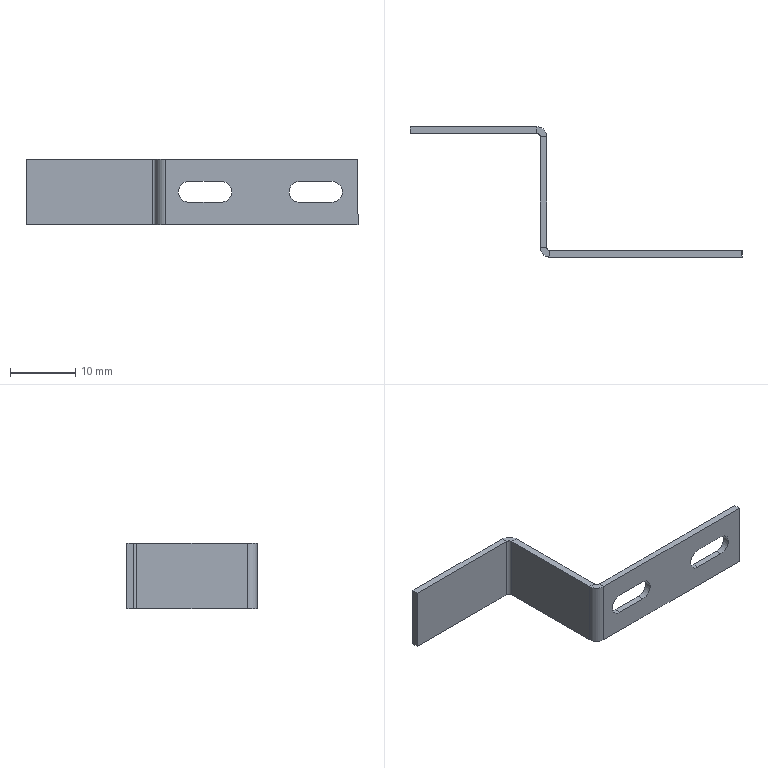Part | SolidWorks | features EdgeFlange 1, FlatPattern 1, ICE 1, SMBaseFlange 1, SheetMetal 1 | 1 solid | 30 faces | box 51 x 20 x 10 mm | volume 643.331 mm3 | plane 22 | cylinder 8 | commonest cylinder face diameters 3.2 x4 1 x2 3 x2
STEP:
#1=CARTESIAN_POINT('',(-1.,17.5,0.));
#2=VERTEX_POINT('',#1);
#3=CARTESIAN_POINT('',(-1.,0.5,0.));
#4=VERTEX_POINT('',#3);
#5=CARTESIAN_POINT('',(-1.,0.,0.));
#6=DIRECTION('',(0.,-1.,0.));
#7=VECTOR('',#6,1000.);
#8=LINE('',#5,#7);
#9=EDGE_CURVE('',#2,#4,#8,.T.);
#10=ORIENTED_EDGE('',*,*,#9,.F.);
#11=CARTESIAN_POINT('',(0.,17.5,0.));
#12=VERTEX_POINT('',#11);
#13=CARTESIAN_POINT('',(-1.,17.5,0.));
#14=DIRECTION('',(1.,0.,0.));
#15=VECTOR('',#14,1000.);
#16=LINE('',#13,#15);
#17=EDGE_CURVE('',#2,#12,#16,.T.);
#18=ORIENTED_EDGE('',*,*,#17,.T.);
#19=CARTESIAN_POINT('',(0.,0.5,0.));
#20=VERTEX_POINT('',#19);
#21=CARTESIAN_POINT('',(0.,0.,0.));
#22=DIRECTION('',(0.,-1.,0.));
#23=VECTOR('',#22,1000.);
#24=LINE('',#21,#23);
#25=EDGE_CURVE('',#12,#20,#24,.T.);
#26=ORIENTED_EDGE('',*,*,#25,.T.);
#27=CARTESIAN_POINT('',(0.,0.5,0.));
#28=DIRECTION('',(-1.,0.,0.));
#29=VECTOR('',#28,1000.);
#30=LINE('',#27,#29);
#31=EDGE_CURVE('',#20,#4,#30,.T.);
#32=ORIENTED_EDGE('',*,*,#31,.T.);
#33=EDGE_LOOP('',(#10,#18,#26,#32));
#34=FACE_OUTER_BOUND('',#33,.T.);
#35=CARTESIAN_POINT('',(0.5,-1.,0.));
#36=DIRECTION('',(0.,0.,-1.));
#37=DIRECTION('',(-1.,0.,0.));
#38=AXIS2_PLACEMENT_3D('',#35,#36,#37);
#39=PLANE('',#38);
#40=ADVANCED_FACE('',(#34),#39,.T.);
#41=ORIENTED_EDGE('',*,*,#25,.F.);
#42=CARTESIAN_POINT('',(0.,17.5,10.));
#43=VERTEX_POINT('',#42);
#44=CARTESIAN_POINT('',(0.,17.5,0.));
#45=DIRECTION('',(0.,0.,1.));
#46=VECTOR('',#45,1000.);
#47=LINE('',#44,#46);
#48=EDGE_CURVE('',#12,#43,#47,.T.);
#49=ORIENTED_EDGE('',*,*,#48,.T.);
#50=CARTESIAN_POINT('',(0.,0.5,10.));
#51=VERTEX_POINT('',#50);
#52=CARTESIAN_POINT('',(0.,0.,10.));
#53=DIRECTION('',(0.,-1.,0.));
#54=VECTOR('',#53,1000.);
#55=LINE('',#52,#54);
#56=EDGE_CURVE('',#43,#51,#55,.T.);
#57=ORIENTED_EDGE('',*,*,#56,.T.);
#58=CARTESIAN_POINT('',(0.,0.5,10.));
#59=DIRECTION('',(0.,0.,-1.));
#60=VECTOR('',#59,1000.);
#61=LINE('',#58,#60);
#62=EDGE_CURVE('',#51,#20,#61,.T.);
#63=ORIENTED_EDGE('',*,*,#62,.T.);
#64=EDGE_LOOP('',(#41,#49,#57,#63));
#65=FACE_OUTER_BOUND('',#64,.T.);
#66=CARTESIAN_POINT('',(0.,0.,10.));
#67=DIRECTION('',(1.,0.,0.));
#68=DIRECTION('',(0.,0.,-1.));
#69=AXIS2_PLACEMENT_3D('',#66,#67,#68);
#70=PLANE('',#69);
#71=ADVANCED_FACE('',(#65),#70,.T.);
#72=CARTESIAN_POINT('',(-1.,17.5,10.));
#73=VERTEX_POINT('',#72);
#74=CARTESIAN_POINT('',(-1.,17.5,0.));
#75=DIRECTION('',(0.,0.,1.));
#76=VECTOR('',#75,1000.);
#77=LINE('',#74,#76);
#78=EDGE_CURVE('',#2,#73,#77,.T.);
#79=ORIENTED_EDGE('',*,*,#78,.F.);
#80=ORIENTED_EDGE('',*,*,#9,.T.);
#81=CARTESIAN_POINT('',(-1.,0.5,10.));
#82=VERTEX_POINT('',#81);
#83=CARTESIAN_POINT('',(-1.,0.5,10.));
#84=DIRECTION('',(0.,0.,-1.));
#85=VECTOR('',#84,1000.);
#86=LINE('',#83,#85);
#87=EDGE_CURVE('',#82,#4,#86,.T.);
#88=ORIENTED_EDGE('',*,*,#87,.F.);
#89=CARTESIAN_POINT('',(-1.,0.,10.));
#90=DIRECTION('',(0.,-1.,0.));
#91=VECTOR('',#90,1000.);
#92=LINE('',#89,#91);
#93=EDGE_CURVE('',#73,#82,#92,.T.);
#94=ORIENTED_EDGE('',*,*,#93,.F.);
#95=EDGE_LOOP('',(#79,#80,#88,#94));
#96=FACE_OUTER_BOUND('',#95,.T.);
#97=CARTESIAN_POINT('',(-1.,0.,10.));
#98=DIRECTION('',(1.,0.,0.));
#99=DIRECTION('',(0.,0.,-1.));
#100=AXIS2_PLACEMENT_3D('',#97,#98,#99);
#101=PLANE('',#100);
#102=ADVANCED_FACE('',(#96),#101,.F.);
#103=CARTESIAN_POINT('',(-1.,17.5,10.));
#104=DIRECTION('',(1.,0.,0.));
#105=VECTOR('',#104,1000.);
#106=LINE('',#103,#105);
#107=EDGE_CURVE('',#73,#43,#106,.T.);
#108=ORIENTED_EDGE('',*,*,#107,.F.);
#109=ORIENTED_EDGE('',*,*,#93,.T.);
#110=CARTESIAN_POINT('',(-1.,0.5,10.));
#111=DIRECTION('',(1.,0.,0.));
#112=VECTOR('',#111,1000.);
#113=LINE('',#110,#112);
#114=EDGE_CURVE('',#82,#51,#113,.T.);
#115=ORIENTED_EDGE('',*,*,#114,.T.);
#116=ORIENTED_EDGE('',*,*,#56,.F.);
#117=EDGE_LOOP('',(#108,#109,#115,#116));
#118=FACE_OUTER_BOUND('',#117,.T.);
#119=CARTESIAN_POINT('',(0.5,0.5,10.));
#120=DIRECTION('',(0.,0.,-1.));
#121=DIRECTION('',(-1.,0.,0.));
#122=AXIS2_PLACEMENT_3D('',#119,#120,#121);
#123=PLANE('',#122);
#124=ADVANCED_FACE('',(#118),#123,.F.);
#125=CARTESIAN_POINT('',(0.5,0.,10.));
#126=VERTEX_POINT('',#125);
#127=CARTESIAN_POINT('',(0.5,-1.,10.));
#128=VERTEX_POINT('',#127);
#129=CARTESIAN_POINT('',(0.5,0.,10.));
#130=DIRECTION('',(0.,-1.,0.));
#131=VECTOR('',#130,1000.);
#132=LINE('',#129,#131);
#133=EDGE_CURVE('',#126,#128,#132,.T.);
#134=ORIENTED_EDGE('',*,*,#133,.F.);
#135=CARTESIAN_POINT('',(0.5,0.5,10.));
#136=DIRECTION('',(0.,0.,1.));
#137=DIRECTION('',(-1.,0.,0.));
#138=AXIS2_PLACEMENT_3D('',#135,#136,#137);
#139=CIRCLE('',#138,0.5);
#140=EDGE_CURVE('',#51,#126,#139,.T.);
#141=ORIENTED_EDGE('',*,*,#140,.F.);
#142=ORIENTED_EDGE('',*,*,#114,.F.);
#143=CARTESIAN_POINT('',(0.5,0.5,10.));
#144=DIRECTION('',(0.,0.,1.));
#145=DIRECTION('',(1.,0.,0.));
#146=AXIS2_PLACEMENT_3D('',#143,#144,#145);
#147=CIRCLE('',#146,1.5);
#148=EDGE_CURVE('',#82,#128,#147,.T.);
#149=ORIENTED_EDGE('',*,*,#148,.T.);
#150=EDGE_LOOP('',(#134,#141,#142,#149));
#151=FACE_OUTER_BOUND('',#150,.T.);
#152=CARTESIAN_POINT('',(0.5,0.,10.));
#153=DIRECTION('',(0.,0.,1.));
#154=DIRECTION('',(1.,0.,0.));
#155=AXIS2_PLACEMENT_3D('',#152,#153,#154);
#156=PLANE('',#155);
#157=ADVANCED_FACE('',(#151),#156,.T.);
#158=CARTESIAN_POINT('',(30.,0.,10.));
#159=VERTEX_POINT('',#158);
#160=CARTESIAN_POINT('',(0.,0.,10.));
#161=DIRECTION('',(1.,0.,0.));
#162=VECTOR('',#161,1000.);
#163=LINE('',#160,#162);
#164=EDGE_CURVE('',#126,#159,#163,.T.);
#165=ORIENTED_EDGE('',*,*,#164,.F.);
#166=ORIENTED_EDGE('',*,*,#133,.T.);
#167=CARTESIAN_POINT('',(30.,-1.,10.));
#168=VERTEX_POINT('',#167);
#169=CARTESIAN_POINT('',(0.,-1.,10.));
#170=DIRECTION('',(1.,0.,0.));
#171=VECTOR('',#170,1000.);
#172=LINE('',#169,#171);
#173=EDGE_CURVE('',#128,#168,#172,.T.);
#174=ORIENTED_EDGE('',*,*,#173,.T.);
#175=CARTESIAN_POINT('',(30.,0.,10.));
#176=DIRECTION('',(0.,-1.,0.));
#177=VECTOR('',#176,1000.);
#178=LINE('',#175,#177);
#179=EDGE_CURVE('',#159,#168,#178,.T.);
#180=ORIENTED_EDGE('',*,*,#179,.F.);
#181=EDGE_LOOP('',(#165,#166,#174,#180));
#182=FACE_OUTER_BOUND('',#181,.T.);
#183=CARTESIAN_POINT('',(-1.,0.5,10.));
#184=DIRECTION('',(0.,0.,1.));
#185=DIRECTION('',(1.,0.,0.));
#186=AXIS2_PLACEMENT_3D('',#183,#184,#185);
#187=PLANE('',#186);
#188=ADVANCED_FACE('',(#182),#187,.T.);
#189=ORIENTED_EDGE('',*,*,#31,.F.);
#190=CARTESIAN_POINT('',(0.5,0.,0.));
#191=VERTEX_POINT('',#190);
#192=CARTESIAN_POINT('',(0.5,0.5,0.));
#193=DIRECTION('',(0.,0.,1.));
#194=DIRECTION('',(-1.,0.,0.));
#195=AXIS2_PLACEMENT_3D('',#192,#193,#194);
#196=CIRCLE('',#195,0.5);
#197=EDGE_CURVE('',#20,#191,#196,.T.);
#198=ORIENTED_EDGE('',*,*,#197,.T.);
#199=CARTESIAN_POINT('',(0.5,-1.,0.));
#200=VERTEX_POINT('',#199);
#201=CARTESIAN_POINT('',(0.5,-1.,0.));
#202=DIRECTION('',(0.,1.,0.));
#203=VECTOR('',#202,1000.);
#204=LINE('',#201,#203);
#205=EDGE_CURVE('',#200,#191,#204,.T.);
#206=ORIENTED_EDGE('',*,*,#205,.F.);
#207=CARTESIAN_POINT('',(0.5,0.5,0.));
#208=DIRECTION('',(0.,0.,1.));
#209=DIRECTION('',(1.,0.,0.));
#210=AXIS2_PLACEMENT_3D('',#207,#208,#209);
#211=CIRCLE('',#210,1.5);
#212=EDGE_CURVE('',#4,#200,#211,.T.);
#213=ORIENTED_EDGE('',*,*,#212,.F.);
#214=EDGE_LOOP('',(#189,#198,#206,#213));
#215=FACE_OUTER_BOUND('',#214,.T.);
#216=CARTESIAN_POINT('',(0.,0.5,0.));
#217=DIRECTION('',(0.,0.,-1.));
#218=DIRECTION('',(-1.,0.,0.));
#219=AXIS2_PLACEMENT_3D('',#216,#217,#218);
#220=PLANE('',#219);
#221=ADVANCED_FACE('',(#215),#220,.T.);
#222=CARTESIAN_POINT('',(26.,-1.,3.43));
#223=VERTEX_POINT('',#222);
#224=CARTESIAN_POINT('',(21.,-1.,3.43));
#225=VERTEX_POINT('',#224);
#226=CARTESIAN_POINT('',(21.,-1.,3.43));
#227=DIRECTION('',(-1.,0.,0.));
#228=VECTOR('',#227,1000.);
#229=LINE('',#226,#228);
#230=EDGE_CURVE('',#223,#225,#229,.T.);
#231=ORIENTED_EDGE('',*,*,#230,.T.);
#232=CARTESIAN_POINT('',(21.,-1.,6.63));
#233=VERTEX_POINT('',#232);
#234=CARTESIAN_POINT('',(21.,-1.,5.03));
#235=DIRECTION('',(0.,1.,0.));
#236=DIRECTION('',(0.,0.,1.));
#237=AXIS2_PLACEMENT_3D('',#234,#235,#236);
#238=CIRCLE('',#237,1.6);
#239=EDGE_CURVE('',#225,#233,#238,.T.);
#240=ORIENTED_EDGE('',*,*,#239,.T.);
#241=CARTESIAN_POINT('',(26.,-1.,6.63));
#242=VERTEX_POINT('',#241);
#243=CARTESIAN_POINT('',(21.,-1.,6.63));
#244=DIRECTION('',(1.,0.,0.));
#245=VECTOR('',#244,1000.);
#246=LINE('',#243,#245);
#247=EDGE_CURVE('',#233,#242,#246,.T.);
#248=ORIENTED_EDGE('',*,*,#247,.T.);
#249=CARTESIAN_POINT('',(26.,-1.,5.03));
#250=DIRECTION('',(0.,1.,0.));
#251=DIRECTION('',(0.,0.,1.));
#252=AXIS2_PLACEMENT_3D('',#249,#250,#251);
#253=CIRCLE('',#252,1.6);
#254=EDGE_CURVE('',#242,#223,#253,.T.);
#255=ORIENTED_EDGE('',*,*,#254,.T.);
#256=EDGE_LOOP('',(#231,#240,#248,#255));
#257=FACE_BOUND('',#256,.T.);
#258=CARTESIAN_POINT('',(9.,-1.,3.43));
#259=VERTEX_POINT('',#258);
#260=CARTESIAN_POINT('',(4.,-1.,3.43));
#261=VERTEX_POINT('',#260);
#262=CARTESIAN_POINT('',(4.,-1.,3.43));
#263=DIRECTION('',(-1.,0.,0.));
#264=VECTOR('',#263,1000.);
#265=LINE('',#262,#264);
#266=EDGE_CURVE('',#259,#261,#265,.T.);
#267=ORIENTED_EDGE('',*,*,#266,.T.);
#268=CARTESIAN_POINT('',(4.,-1.,6.63));
#269=VERTEX_POINT('',#268);
#270=CARTESIAN_POINT('',(4.,-1.,5.03));
#271=DIRECTION('',(0.,1.,0.));
#272=DIRECTION('',(0.,0.,1.));
#273=AXIS2_PLACEMENT_3D('',#270,#271,#272);
#274=CIRCLE('',#273,1.6);
#275=EDGE_CURVE('',#261,#269,#274,.T.);
#276=ORIENTED_EDGE('',*,*,#275,.T.);
#277=CARTESIAN_POINT('',(9.,-1.,6.63));
#278=VERTEX_POINT('',#277);
#279=CARTESIAN_POINT('',(4.,-1.,6.63));
#280=DIRECTION('',(1.,0.,0.));
#281=VECTOR('',#280,1000.);
#282=LINE('',#279,#281);
#283=EDGE_CURVE('',#269,#278,#282,.T.);
#284=ORIENTED_EDGE('',*,*,#283,.T.);
#285=CARTESIAN_POINT('',(9.,-1.,5.03));
#286=DIRECTION('',(0.,1.,0.));
#287=DIRECTION('',(0.,0.,1.));
#288=AXIS2_PLACEMENT_3D('',#285,#286,#287);
#289=CIRCLE('',#288,1.6);
#290=EDGE_CURVE('',#278,#259,#289,.T.);
#291=ORIENTED_EDGE('',*,*,#290,.T.);
#292=EDGE_LOOP('',(#267,#276,#284,#291));
#293=FACE_BOUND('',#292,.T.);
#294=CARTESIAN_POINT('',(30.,-1.,0.));
#295=VERTEX_POINT('',#294);
#296=CARTESIAN_POINT('',(0.,-1.,0.));
#297=DIRECTION('',(1.,0.,0.));
#298=VECTOR('',#297,1000.);
#299=LINE('',#296,#298);
#300=EDGE_CURVE('',#200,#295,#299,.T.);
#301=ORIENTED_EDGE('',*,*,#300,.T.);
#302=CARTESIAN_POINT('',(30.,-1.,10.));
#303=DIRECTION('',(0.,0.,-1.));
#304=VECTOR('',#303,1000.);
#305=LINE('',#302,#304);
#306=EDGE_CURVE('',#168,#295,#305,.T.);
#307=ORIENTED_EDGE('',*,*,#306,.F.);
#308=ORIENTED_EDGE('',*,*,#173,.F.);
#309=CARTESIAN_POINT('',(0.5,-1.,10.));
#310=DIRECTION('',(0.,0.,-1.));
#311=VECTOR('',#310,1000.);
#312=LINE('',#309,#311);
#313=EDGE_CURVE('',#128,#200,#312,.T.);
#314=ORIENTED_EDGE('',*,*,#313,.T.);
#315=EDGE_LOOP('',(#301,#307,#308,#314));
#316=FACE_OUTER_BOUND('',#315,.T.);
#317=CARTESIAN_POINT('',(0.,-1.,10.));
#318=DIRECTION('',(0.,1.,0.));
#319=DIRECTION('',(0.,0.,1.));
#320=AXIS2_PLACEMENT_3D('',#317,#318,#319);
#321=PLANE('',#320);
#322=ADVANCED_FACE('',(#257,#293,#316),#321,.F.);
#323=CARTESIAN_POINT('',(30.,0.,0.));
#324=VERTEX_POINT('',#323);
#325=CARTESIAN_POINT('',(30.,0.,0.));
#326=DIRECTION('',(0.,-1.,0.));
#327=VECTOR('',#326,1000.);
#328=LINE('',#325,#327);
#329=EDGE_CURVE('',#324,#295,#328,.T.);
#330=ORIENTED_EDGE('',*,*,#329,.F.);
#331=CARTESIAN_POINT('',(30.,0.,10.));
#332=DIRECTION('',(0.,0.,-1.));
#333=VECTOR('',#332,1000.);
#334=LINE('',#331,#333);
#335=EDGE_CURVE('',#159,#324,#334,.T.);
#336=ORIENTED_EDGE('',*,*,#335,.F.);
#337=ORIENTED_EDGE('',*,*,#179,.T.);
#338=ORIENTED_EDGE('',*,*,#306,.T.);
#339=EDGE_LOOP('',(#330,#336,#337,#338));
#340=FACE_OUTER_BOUND('',#339,.T.);
#341=CARTESIAN_POINT('',(30.,0.,10.));
#342=DIRECTION('',(1.,0.,0.));
#343=DIRECTION('',(0.,0.,-1.));
#344=AXIS2_PLACEMENT_3D('',#341,#342,#343);
#345=PLANE('',#344);
#346=ADVANCED_FACE('',(#340),#345,.T.);
#347=CARTESIAN_POINT('',(21.,0.,3.43));
#348=VERTEX_POINT('',#347);
#349=CARTESIAN_POINT('',(21.,0.,6.63));
#350=VERTEX_POINT('',#349);
#351=CARTESIAN_POINT('',(21.,0.,5.03));
#352=DIRECTION('',(0.,1.,0.));
#353=DIRECTION('',(0.,0.,1.));
#354=AXIS2_PLACEMENT_3D('',#351,#352,#353);
#355=CIRCLE('',#354,1.6);
#356=EDGE_CURVE('',#348,#350,#355,.T.);
#357=ORIENTED_EDGE('',*,*,#356,.F.);
#358=CARTESIAN_POINT('',(26.,0.,3.43));
#359=VERTEX_POINT('',#358);
#360=CARTESIAN_POINT('',(21.,0.,3.43));
#361=DIRECTION('',(-1.,0.,0.));
#362=VECTOR('',#361,1000.);
#363=LINE('',#360,#362);
#364=EDGE_CURVE('',#359,#348,#363,.T.);
#365=ORIENTED_EDGE('',*,*,#364,.F.);
#366=CARTESIAN_POINT('',(26.,0.,6.63));
#367=VERTEX_POINT('',#366);
#368=CARTESIAN_POINT('',(26.,0.,5.03));
#369=DIRECTION('',(0.,1.,0.));
#370=DIRECTION('',(0.,0.,1.));
#371=AXIS2_PLACEMENT_3D('',#368,#369,#370);
#372=CIRCLE('',#371,1.6);
#373=EDGE_CURVE('',#367,#359,#372,.T.);
#374=ORIENTED_EDGE('',*,*,#373,.F.);
#375=CARTESIAN_POINT('',(21.,0.,6.63));
#376=DIRECTION('',(1.,0.,0.));
#377=VECTOR('',#376,1000.);
#378=LINE('',#375,#377);
#379=EDGE_CURVE('',#350,#367,#378,.T.);
#380=ORIENTED_EDGE('',*,*,#379,.F.);
#381=EDGE_LOOP('',(#357,#365,#374,#380));
#382=FACE_BOUND('',#381,.T.);
#383=CARTESIAN_POINT('',(4.,0.,3.43));
#384=VERTEX_POINT('',#383);
#385=CARTESIAN_POINT('',(4.,0.,6.63));
#386=VERTEX_POINT('',#385);
#387=CARTESIAN_POINT('',(4.,0.,5.03));
#388=DIRECTION('',(0.,1.,0.));
#389=DIRECTION('',(0.,0.,1.));
#390=AXIS2_PLACEMENT_3D('',#387,#388,#389);
#391=CIRCLE('',#390,1.6);
#392=EDGE_CURVE('',#384,#386,#391,.T.);
#393=ORIENTED_EDGE('',*,*,#392,.F.);
#394=CARTESIAN_POINT('',(9.,0.,3.43));
#395=VERTEX_POINT('',#394);
#396=CARTESIAN_POINT('',(4.,0.,3.43));
#397=DIRECTION('',(-1.,0.,0.));
#398=VECTOR('',#397,1000.);
#399=LINE('',#396,#398);
#400=EDGE_CURVE('',#395,#384,#399,.T.);
#401=ORIENTED_EDGE('',*,*,#400,.F.);
#402=CARTESIAN_POINT('',(9.,0.,6.63));
#403=VERTEX_POINT('',#402);
#404=CARTESIAN_POINT('',(9.,0.,5.03));
#405=DIRECTION('',(0.,1.,0.));
#406=DIRECTION('',(0.,0.,1.));
#407=AXIS2_PLACEMENT_3D('',#404,#405,#406);
#408=CIRCLE('',#407,1.6);
#409=EDGE_CURVE('',#403,#395,#408,.T.);
#410=ORIENTED_EDGE('',*,*,#409,.F.);
#411=CARTESIAN_POINT('',(4.,0.,6.63));
#412=DIRECTION('',(1.,0.,0.));
#413=VECTOR('',#412,1000.);
#414=LINE('',#411,#413);
#415=EDGE_CURVE('',#386,#403,#414,.T.);
#416=ORIENTED_EDGE('',*,*,#415,.F.);
#417=EDGE_LOOP('',(#393,#401,#410,#416));
#418=FACE_BOUND('',#417,.T.);
#419=CARTESIAN_POINT('',(0.,0.,0.));
#420=DIRECTION('',(1.,0.,0.));
#421=VECTOR('',#420,1000.);
#422=LINE('',#419,#421);
#423=EDGE_CURVE('',#191,#324,#422,.T.);
#424=ORIENTED_EDGE('',*,*,#423,.F.);
#425=CARTESIAN_POINT('',(0.5,0.,10.));
#426=DIRECTION('',(0.,0.,-1.));
#427=VECTOR('',#426,1000.);
#428=LINE('',#425,#427);
#429=EDGE_CURVE('',#126,#191,#428,.T.);
#430=ORIENTED_EDGE('',*,*,#429,.F.);
#431=ORIENTED_EDGE('',*,*,#164,.T.);
#432=ORIENTED_EDGE('',*,*,#335,.T.);
#433=EDGE_LOOP('',(#424,#430,#431,#432));
#434=FACE_OUTER_BOUND('',#433,.T.);
#435=CARTESIAN_POINT('',(0.,0.,10.));
#436=DIRECTION('',(0.,1.,0.));
#437=DIRECTION('',(0.,0.,1.));
#438=AXIS2_PLACEMENT_3D('',#435,#436,#437);
#439=PLANE('',#438);
#440=ADVANCED_FACE('',(#382,#418,#434),#439,.T.);
#441=ORIENTED_EDGE('',*,*,#197,.F.);
#442=ORIENTED_EDGE('',*,*,#62,.F.);
#443=ORIENTED_EDGE('',*,*,#140,.T.);
#444=ORIENTED_EDGE('',*,*,#429,.T.);
#445=EDGE_LOOP('',(#441,#442,#443,#444));
#446=FACE_OUTER_BOUND('',#445,.T.);
#447=CARTESIAN_POINT('',(0.5,0.5,10.));
#448=DIRECTION('',(0.,0.,-1.));
#449=DIRECTION('',(-1.,0.,0.));
#450=AXIS2_PLACEMENT_3D('',#447,#448,#449);
#451=CYLINDRICAL_SURFACE('',#450,0.5);
#452=ADVANCED_FACE('',(#446),#451,.F.);
#453=ORIENTED_EDGE('',*,*,#212,.T.);
#454=ORIENTED_EDGE('',*,*,#313,.F.);
#455=ORIENTED_EDGE('',*,*,#148,.F.);
#456=ORIENTED_EDGE('',*,*,#87,.T.);
#457=EDGE_LOOP('',(#453,#454,#455,#456));
#458=FACE_OUTER_BOUND('',#457,.T.);
#459=CARTESIAN_POINT('',(0.5,0.5,10.));
#460=DIRECTION('',(0.,0.,-1.));
#461=DIRECTION('',(-1.,0.,0.));
#462=AXIS2_PLACEMENT_3D('',#459,#460,#461);
#463=CYLINDRICAL_SURFACE('',#462,1.5);
#464=ADVANCED_FACE('',(#458),#463,.T.);
#465=ORIENTED_EDGE('',*,*,#300,.F.);
#466=ORIENTED_EDGE('',*,*,#205,.T.);
#467=ORIENTED_EDGE('',*,*,#423,.T.);
#468=ORIENTED_EDGE('',*,*,#329,.T.);
#469=EDGE_LOOP('',(#465,#466,#467,#468));
#470=FACE_OUTER_BOUND('',#469,.T.);
#471=CARTESIAN_POINT('',(0.5,0.5,0.));
#472=DIRECTION('',(0.,0.,-1.));
#473=DIRECTION('',(-1.,0.,0.));
#474=AXIS2_PLACEMENT_3D('',#471,#472,#473);
#475=PLANE('',#474);
#476=ADVANCED_FACE('',(#470),#475,.T.);
#477=CARTESIAN_POINT('',(-1.5,18.,10.));
#478=VERTEX_POINT('',#477);
#479=CARTESIAN_POINT('',(-1.5,19.,10.));
#480=VERTEX_POINT('',#479);
#481=CARTESIAN_POINT('',(-1.5,18.,10.));
#482=DIRECTION('',(0.,1.,0.));
#483=VECTOR('',#482,1000.);
#484=LINE('',#481,#483);
#485=EDGE_CURVE('',#478,#480,#484,.T.);
#486=ORIENTED_EDGE('',*,*,#485,.F.);
#487=CARTESIAN_POINT('',(-1.5,17.5,10.));
#488=DIRECTION('',(0.,0.,1.));
#489=DIRECTION('',(-1.,0.,0.));
#490=AXIS2_PLACEMENT_3D('',#487,#488,#489);
#491=CIRCLE('',#490,0.5);
#492=EDGE_CURVE('',#73,#478,#491,.T.);
#493=ORIENTED_EDGE('',*,*,#492,.F.);
#494=ORIENTED_EDGE('',*,*,#107,.T.);
#495=CARTESIAN_POINT('',(-1.5,17.5,10.));
#496=DIRECTION('',(0.,0.,1.));
#497=DIRECTION('',(-1.,0.,0.));
#498=AXIS2_PLACEMENT_3D('',#495,#496,#497);
#499=CIRCLE('',#498,1.5);
#500=EDGE_CURVE('',#43,#480,#499,.T.);
#501=ORIENTED_EDGE('',*,*,#500,.T.);
#502=EDGE_LOOP('',(#486,#493,#494,#501));
#503=FACE_OUTER_BOUND('',#502,.T.);
#504=CARTESIAN_POINT('',(-1.5,17.5,10.));
#505=DIRECTION('',(0.,0.,1.));
#506=DIRECTION('',(1.,0.,0.));
#507=AXIS2_PLACEMENT_3D('',#504,#505,#506);
#508=PLANE('',#507);
#509=ADVANCED_FACE('',(#503),#508,.T.);
#510=CARTESIAN_POINT('',(-1.5,18.,0.));
#511=VERTEX_POINT('',#510);
#512=CARTESIAN_POINT('',(-1.5,17.5,0.));
#513=DIRECTION('',(0.,0.,-1.));
#514=DIRECTION('',(-1.,0.,0.));
#515=AXIS2_PLACEMENT_3D('',#512,#513,#514);
#516=CIRCLE('',#515,0.5);
#517=EDGE_CURVE('',#511,#2,#516,.T.);
#518=ORIENTED_EDGE('',*,*,#517,.F.);
#519=CARTESIAN_POINT('',(-1.5,19.,0.));
#520=VERTEX_POINT('',#519);
#521=CARTESIAN_POINT('',(-1.5,18.,0.));
#522=DIRECTION('',(0.,1.,0.));
#523=VECTOR('',#522,1000.);
#524=LINE('',#521,#523);
#525=EDGE_CURVE('',#511,#520,#524,.T.);
#526=ORIENTED_EDGE('',*,*,#525,.T.);
#527=CARTESIAN_POINT('',(-1.5,17.5,0.));
#528=DIRECTION('',(0.,0.,-1.));
#529=DIRECTION('',(-1.,0.,0.));
#530=AXIS2_PLACEMENT_3D('',#527,#528,#529);
#531=CIRCLE('',#530,1.5);
#532=EDGE_CURVE('',#520,#12,#531,.T.);
#533=ORIENTED_EDGE('',*,*,#532,.T.);
#534=ORIENTED_EDGE('',*,*,#17,.F.);
#535=EDGE_LOOP('',(#518,#526,#533,#534));
#536=FACE_OUTER_BOUND('',#535,.T.);
#537=CARTESIAN_POINT('',(-1.5,17.5,0.));
#538=DIRECTION('',(0.,0.,1.));
#539=DIRECTION('',(1.,0.,0.));
#540=AXIS2_PLACEMENT_3D('',#537,#538,#539);
#541=PLANE('',#540);
#542=ADVANCED_FACE('',(#536),#541,.F.);
#543=ORIENTED_EDGE('',*,*,#48,.F.);
#544=ORIENTED_EDGE('',*,*,#532,.F.);
#545=CARTESIAN_POINT('',(-1.5,19.,0.));
#546=DIRECTION('',(0.,0.,1.));
#547=VECTOR('',#546,1000.);
#548=LINE('',#545,#547);
#549=EDGE_CURVE('',#520,#480,#548,.T.);
#550=ORIENTED_EDGE('',*,*,#549,.T.);
#551=ORIENTED_EDGE('',*,*,#500,.F.);
#552=EDGE_LOOP('',(#543,#544,#550,#551));
#553=FACE_OUTER_BOUND('',#552,.T.);
#554=CARTESIAN_POINT('',(-1.5,17.5,0.));
#555=DIRECTION('',(0.,0.,-1.));
#556=DIRECTION('',(0.,1.,0.));
#557=AXIS2_PLACEMENT_3D('',#554,#555,#556);
#558=CYLINDRICAL_SURFACE('',#557,1.5);
#559=ADVANCED_FACE('',(#553),#558,.T.);
#560=ORIENTED_EDGE('',*,*,#78,.T.);
#561=ORIENTED_EDGE('',*,*,#492,.T.);
#562=CARTESIAN_POINT('',(-1.5,18.,10.));
#563=DIRECTION('',(0.,0.,-1.));
#564=VECTOR('',#563,1000.);
#565=LINE('',#562,#564);
#566=EDGE_CURVE('',#478,#511,#565,.T.);
#567=ORIENTED_EDGE('',*,*,#566,.T.);
#568=ORIENTED_EDGE('',*,*,#517,.T.);
#569=EDGE_LOOP('',(#560,#561,#567,#568));
#570=FACE_OUTER_BOUND('',#569,.T.);
#571=CARTESIAN_POINT('',(-1.5,17.5,0.));
#572=DIRECTION('',(0.,0.,-1.));
#573=DIRECTION('',(0.,1.,0.));
#574=AXIS2_PLACEMENT_3D('',#571,#572,#573);
#575=CYLINDRICAL_SURFACE('',#574,0.5);
#576=ADVANCED_FACE('',(#570),#575,.F.);
#577=ORIENTED_EDGE('',*,*,#485,.T.);
#578=CARTESIAN_POINT('',(-21.,19.,10.));
#579=VERTEX_POINT('',#578);
#580=CARTESIAN_POINT('',(-1.,19.,10.));
#581=DIRECTION('',(1.,0.,0.));
#582=VECTOR('',#581,1000.);
#583=LINE('',#580,#582);
#584=EDGE_CURVE('',#579,#480,#583,.T.);
#585=ORIENTED_EDGE('',*,*,#584,.F.);
#586=CARTESIAN_POINT('',(-21.,18.,10.));
#587=VERTEX_POINT('',#586);
#588=CARTESIAN_POINT('',(-21.,19.,10.));
#589=DIRECTION('',(0.,-1.,0.));
#590=VECTOR('',#589,1000.);
#591=LINE('',#588,#590);
#592=EDGE_CURVE('',#579,#587,#591,.T.);
#593=ORIENTED_EDGE('',*,*,#592,.T.);
#594=CARTESIAN_POINT('',(-1.,18.,10.));
#595=DIRECTION('',(1.,0.,0.));
#596=VECTOR('',#595,1000.);
#597=LINE('',#594,#596);
#598=EDGE_CURVE('',#587,#478,#597,.T.);
#599=ORIENTED_EDGE('',*,*,#598,.T.);
#600=EDGE_LOOP('',(#577,#585,#593,#599));
#601=FACE_OUTER_BOUND('',#600,.T.);
#602=CARTESIAN_POINT('',(-1.,19.,10.));
#603=DIRECTION('',(0.,0.,-1.));
#604=DIRECTION('',(-1.,0.,0.));
#605=AXIS2_PLACEMENT_3D('',#602,#603,#604);
#606=PLANE('',#605);
#607=ADVANCED_FACE('',(#601),#606,.F.);
#608=ORIENTED_EDGE('',*,*,#525,.F.);
#609=CARTESIAN_POINT('',(-21.,18.,0.));
#610=VERTEX_POINT('',#609);
#611=CARTESIAN_POINT('',(-21.,18.,0.));
#612=DIRECTION('',(-1.,0.,0.));
#613=VECTOR('',#612,1000.);
#614=LINE('',#611,#613);
#615=EDGE_CURVE('',#511,#610,#614,.T.);
#616=ORIENTED_EDGE('',*,*,#615,.T.);
#617=CARTESIAN_POINT('',(-21.,19.,0.));
#618=VERTEX_POINT('',#617);
#619=CARTESIAN_POINT('',(-21.,19.,0.));
#620=DIRECTION('',(0.,-1.,0.));
#621=VECTOR('',#620,1000.);
#622=LINE('',#619,#621);
#623=EDGE_CURVE('',#618,#610,#622,.T.);
#624=ORIENTED_EDGE('',*,*,#623,.F.);
#625=CARTESIAN_POINT('',(-21.,19.,0.));
#626=DIRECTION('',(-1.,0.,0.));
#627=VECTOR('',#626,1000.);
#628=LINE('',#625,#627);
#629=EDGE_CURVE('',#520,#618,#628,.T.);
#630=ORIENTED_EDGE('',*,*,#629,.F.);
#631=EDGE_LOOP('',(#608,#616,#624,#630));
#632=FACE_OUTER_BOUND('',#631,.T.);
#633=CARTESIAN_POINT('',(-21.,19.,0.));
#634=DIRECTION('',(0.,0.,1.));
#635=DIRECTION('',(1.,0.,0.));
#636=AXIS2_PLACEMENT_3D('',#633,#634,#635);
#637=PLANE('',#636);
#638=ADVANCED_FACE('',(#632),#637,.F.);
#639=ORIENTED_EDGE('',*,*,#549,.F.);
#640=ORIENTED_EDGE('',*,*,#629,.T.);
#641=CARTESIAN_POINT('',(-21.,19.,10.));
#642=DIRECTION('',(0.,0.,1.));
#643=VECTOR('',#642,1000.);
#644=LINE('',#641,#643);
#645=EDGE_CURVE('',#618,#579,#644,.T.);
#646=ORIENTED_EDGE('',*,*,#645,.T.);
#647=ORIENTED_EDGE('',*,*,#584,.T.);
#648=EDGE_LOOP('',(#639,#640,#646,#647));
#649=FACE_OUTER_BOUND('',#648,.T.);
#650=CARTESIAN_POINT('',(0.,19.,0.));
#651=DIRECTION('',(0.,-1.,0.));
#652=DIRECTION('',(1.,0.,0.));
#653=AXIS2_PLACEMENT_3D('',#650,#651,#652);
#654=PLANE('',#653);
#655=ADVANCED_FACE('',(#649),#654,.F.);
#656=ORIENTED_EDGE('',*,*,#615,.F.);
#657=ORIENTED_EDGE('',*,*,#566,.F.);
#658=ORIENTED_EDGE('',*,*,#598,.F.);
#659=CARTESIAN_POINT('',(-21.,18.,10.));
#660=DIRECTION('',(0.,0.,1.));
#661=VECTOR('',#660,1000.);
#662=LINE('',#659,#661);
#663=EDGE_CURVE('',#610,#587,#662,.T.);
#664=ORIENTED_EDGE('',*,*,#663,.F.);
#665=EDGE_LOOP('',(#656,#657,#658,#664));
#666=FACE_OUTER_BOUND('',#665,.T.);
#667=CARTESIAN_POINT('',(0.,18.,0.));
#668=DIRECTION('',(0.,-1.,0.));
#669=DIRECTION('',(1.,0.,0.));
#670=AXIS2_PLACEMENT_3D('',#667,#668,#669);
#671=PLANE('',#670);
#672=ADVANCED_FACE('',(#666),#671,.T.);
#673=ORIENTED_EDGE('',*,*,#663,.T.);
#674=ORIENTED_EDGE('',*,*,#592,.F.);
#675=ORIENTED_EDGE('',*,*,#645,.F.);
#676=ORIENTED_EDGE('',*,*,#623,.T.);
#677=EDGE_LOOP('',(#673,#674,#675,#676));
#678=FACE_OUTER_BOUND('',#677,.T.);
#679=CARTESIAN_POINT('',(-21.,19.,10.));
#680=DIRECTION('',(1.,0.,0.));
#681=DIRECTION('',(0.,1.,0.));
#682=AXIS2_PLACEMENT_3D('',#679,#680,#681);
#683=PLANE('',#682);
#684=ADVANCED_FACE('',(#678),#683,.F.);
#685=ORIENTED_EDGE('',*,*,#392,.T.);
#686=CARTESIAN_POINT('',(4.,-1.,6.63));
#687=DIRECTION('',(0.,1.,0.));
#688=VECTOR('',#687,1000.);
#689=LINE('',#686,#688);
#690=EDGE_CURVE('',#269,#386,#689,.T.);
#691=ORIENTED_EDGE('',*,*,#690,.F.);
#692=ORIENTED_EDGE('',*,*,#275,.F.);
#693=CARTESIAN_POINT('',(4.,-1.,3.43));
#694=DIRECTION('',(0.,1.,0.));
#695=VECTOR('',#694,1000.);
#696=LINE('',#693,#695);
#697=EDGE_CURVE('',#261,#384,#696,.T.);
#698=ORIENTED_EDGE('',*,*,#697,.T.);
#699=EDGE_LOOP('',(#685,#691,#692,#698));
#700=FACE_OUTER_BOUND('',#699,.T.);
#701=CARTESIAN_POINT('',(4.,-1.,5.03));
#702=DIRECTION('',(0.,1.,0.));
#703=DIRECTION('',(0.,0.,1.));
#704=AXIS2_PLACEMENT_3D('',#701,#702,#703);
#705=CYLINDRICAL_SURFACE('',#704,1.6);
#706=ADVANCED_FACE('',(#700),#705,.F.);
#707=ORIENTED_EDGE('',*,*,#400,.T.);
#708=ORIENTED_EDGE('',*,*,#697,.F.);
#709=ORIENTED_EDGE('',*,*,#266,.F.);
#710=CARTESIAN_POINT('',(9.,-1.,3.43));
#711=DIRECTION('',(0.,1.,0.));
#712=VECTOR('',#711,1000.);
#713=LINE('',#710,#712);
#714=EDGE_CURVE('',#259,#395,#713,.T.);
#715=ORIENTED_EDGE('',*,*,#714,.T.);
#716=EDGE_LOOP('',(#707,#708,#709,#715));
#717=FACE_OUTER_BOUND('',#716,.T.);
#718=CARTESIAN_POINT('',(4.,-1.,3.43));
#719=DIRECTION('',(0.,0.,-1.));
#720=DIRECTION('',(-1.,0.,0.));
#721=AXIS2_PLACEMENT_3D('',#718,#719,#720);
#722=PLANE('',#721);
#723=ADVANCED_FACE('',(#717),#722,.F.);
#724=ORIENTED_EDGE('',*,*,#409,.T.);
#725=ORIENTED_EDGE('',*,*,#714,.F.);
#726=ORIENTED_EDGE('',*,*,#290,.F.);
#727=CARTESIAN_POINT('',(9.,-1.,6.63));
#728=DIRECTION('',(0.,1.,0.));
#729=VECTOR('',#728,1000.);
#730=LINE('',#727,#729);
#731=EDGE_CURVE('',#278,#403,#730,.T.);
#732=ORIENTED_EDGE('',*,*,#731,.T.);
#733=EDGE_LOOP('',(#724,#725,#726,#732));
#734=FACE_OUTER_BOUND('',#733,.T.);
#735=CARTESIAN_POINT('',(9.,-1.,5.03));
#736=DIRECTION('',(0.,1.,0.));
#737=DIRECTION('',(0.,0.,1.));
#738=AXIS2_PLACEMENT_3D('',#735,#736,#737);
#739=CYLINDRICAL_SURFACE('',#738,1.6);
#740=ADVANCED_FACE('',(#734),#739,.F.);
#741=ORIENTED_EDGE('',*,*,#415,.T.);
#742=ORIENTED_EDGE('',*,*,#731,.F.);
#743=ORIENTED_EDGE('',*,*,#283,.F.);
#744=ORIENTED_EDGE('',*,*,#690,.T.);
#745=EDGE_LOOP('',(#741,#742,#743,#744));
#746=FACE_OUTER_BOUND('',#745,.T.);
#747=CARTESIAN_POINT('',(4.,-1.,6.63));
#748=DIRECTION('',(0.,0.,1.));
#749=DIRECTION('',(1.,0.,0.));
#750=AXIS2_PLACEMENT_3D('',#747,#748,#749);
#751=PLANE('',#750);
#752=ADVANCED_FACE('',(#746),#751,.F.);
#753=ORIENTED_EDGE('',*,*,#356,.T.);
#754=CARTESIAN_POINT('',(21.,-1.,6.63));
#755=DIRECTION('',(0.,1.,0.));
#756=VECTOR('',#755,1000.);
#757=LINE('',#754,#756);
#758=EDGE_CURVE('',#233,#350,#757,.T.);
#759=ORIENTED_EDGE('',*,*,#758,.F.);
#760=ORIENTED_EDGE('',*,*,#239,.F.);
#761=CARTESIAN_POINT('',(21.,-1.,3.43));
#762=DIRECTION('',(0.,1.,0.));
#763=VECTOR('',#762,1000.);
#764=LINE('',#761,#763);
#765=EDGE_CURVE('',#225,#348,#764,.T.);
#766=ORIENTED_EDGE('',*,*,#765,.T.);
#767=EDGE_LOOP('',(#753,#759,#760,#766));
#768=FACE_OUTER_BOUND('',#767,.T.);
#769=CARTESIAN_POINT('',(21.,-1.,5.03));
#770=DIRECTION('',(0.,1.,0.));
#771=DIRECTION('',(0.,0.,1.));
#772=AXIS2_PLACEMENT_3D('',#769,#770,#771);
#773=CYLINDRICAL_SURFACE('',#772,1.6);
#774=ADVANCED_FACE('',(#768),#773,.F.);
#775=ORIENTED_EDGE('',*,*,#364,.T.);
#776=ORIENTED_EDGE('',*,*,#765,.F.);
#777=ORIENTED_EDGE('',*,*,#230,.F.);
#778=CARTESIAN_POINT('',(26.,-1.,3.43));
#779=DIRECTION('',(0.,1.,0.));
#780=VECTOR('',#779,1000.);
#781=LINE('',#778,#780);
#782=EDGE_CURVE('',#223,#359,#781,.T.);
#783=ORIENTED_EDGE('',*,*,#782,.T.);
#784=EDGE_LOOP('',(#775,#776,#777,#783));
#785=FACE_OUTER_BOUND('',#784,.T.);
#786=CARTESIAN_POINT('',(21.,-1.,3.43));
#787=DIRECTION('',(0.,0.,-1.));
#788=DIRECTION('',(-1.,0.,0.));
#789=AXIS2_PLACEMENT_3D('',#786,#787,#788);
#790=PLANE('',#789);
#791=ADVANCED_FACE('',(#785),#790,.F.);
#792=ORIENTED_EDGE('',*,*,#373,.T.);
#793=ORIENTED_EDGE('',*,*,#782,.F.);
#794=ORIENTED_EDGE('',*,*,#254,.F.);
#795=CARTESIAN_POINT('',(26.,-1.,6.63));
#796=DIRECTION('',(0.,1.,0.));
#797=VECTOR('',#796,1000.);
#798=LINE('',#795,#797);
#799=EDGE_CURVE('',#242,#367,#798,.T.);
#800=ORIENTED_EDGE('',*,*,#799,.T.);
#801=EDGE_LOOP('',(#792,#793,#794,#800));
#802=FACE_OUTER_BOUND('',#801,.T.);
#803=CARTESIAN_POINT('',(26.,-1.,5.03));
#804=DIRECTION('',(0.,1.,0.));
#805=DIRECTION('',(0.,0.,1.));
#806=AXIS2_PLACEMENT_3D('',#803,#804,#805);
#807=CYLINDRICAL_SURFACE('',#806,1.6);
#808=ADVANCED_FACE('',(#802),#807,.F.);
#809=ORIENTED_EDGE('',*,*,#379,.T.);
#810=ORIENTED_EDGE('',*,*,#799,.F.);
#811=ORIENTED_EDGE('',*,*,#247,.F.);
#812=ORIENTED_EDGE('',*,*,#758,.T.);
#813=EDGE_LOOP('',(#809,#810,#811,#812));
#814=FACE_OUTER_BOUND('',#813,.T.);
#815=CARTESIAN_POINT('',(21.,-1.,6.63));
#816=DIRECTION('',(0.,0.,1.));
#817=DIRECTION('',(1.,0.,0.));
#818=AXIS2_PLACEMENT_3D('',#815,#816,#817);
#819=PLANE('',#818);
#820=ADVANCED_FACE('',(#814),#819,.F.);
#821=CLOSED_SHELL('',(#40,#71,#102,#124,#157,#188,#221,#322,#346,#440,#452,#464,#476,#509,#542,#559,#576,#607,#638,#655,#672,#684,#706,#723,#740,#752,#774,#791,#808,#820));
#822=MANIFOLD_SOLID_BREP('',#821);
#823=CARTESIAN_POINT('',(0.,0.,0.));
#824=DIRECTION('',(0.,0.,1.));
#825=DIRECTION('',(1.,0.,0.));
#826=AXIS2_PLACEMENT_3D('',#823,#824,#825);
#827=(LENGTH_UNIT()NAMED_UNIT(*)SI_UNIT(.MILLI.,.METRE.));
#828=UNCERTAINTY_MEASURE_WITH_UNIT(LENGTH_MEASURE(0.00001),#827,'','');
#829=(NAMED_UNIT(*)PLANE_ANGLE_UNIT()SI_UNIT($,.RADIAN.));
#830=(NAMED_UNIT(*)SI_UNIT($,.STERADIAN.)SOLID_ANGLE_UNIT());
#831=(GEOMETRIC_REPRESENTATION_CONTEXT(3)GLOBAL_UNCERTAINTY_ASSIGNED_CONTEXT((#828))GLOBAL_UNIT_ASSIGNED_CONTEXT((#827,#829,#830))REPRESENTATION_CONTEXT('',''));
#832=ADVANCED_BREP_SHAPE_REPRESENTATION('',(#822,#826),#831);